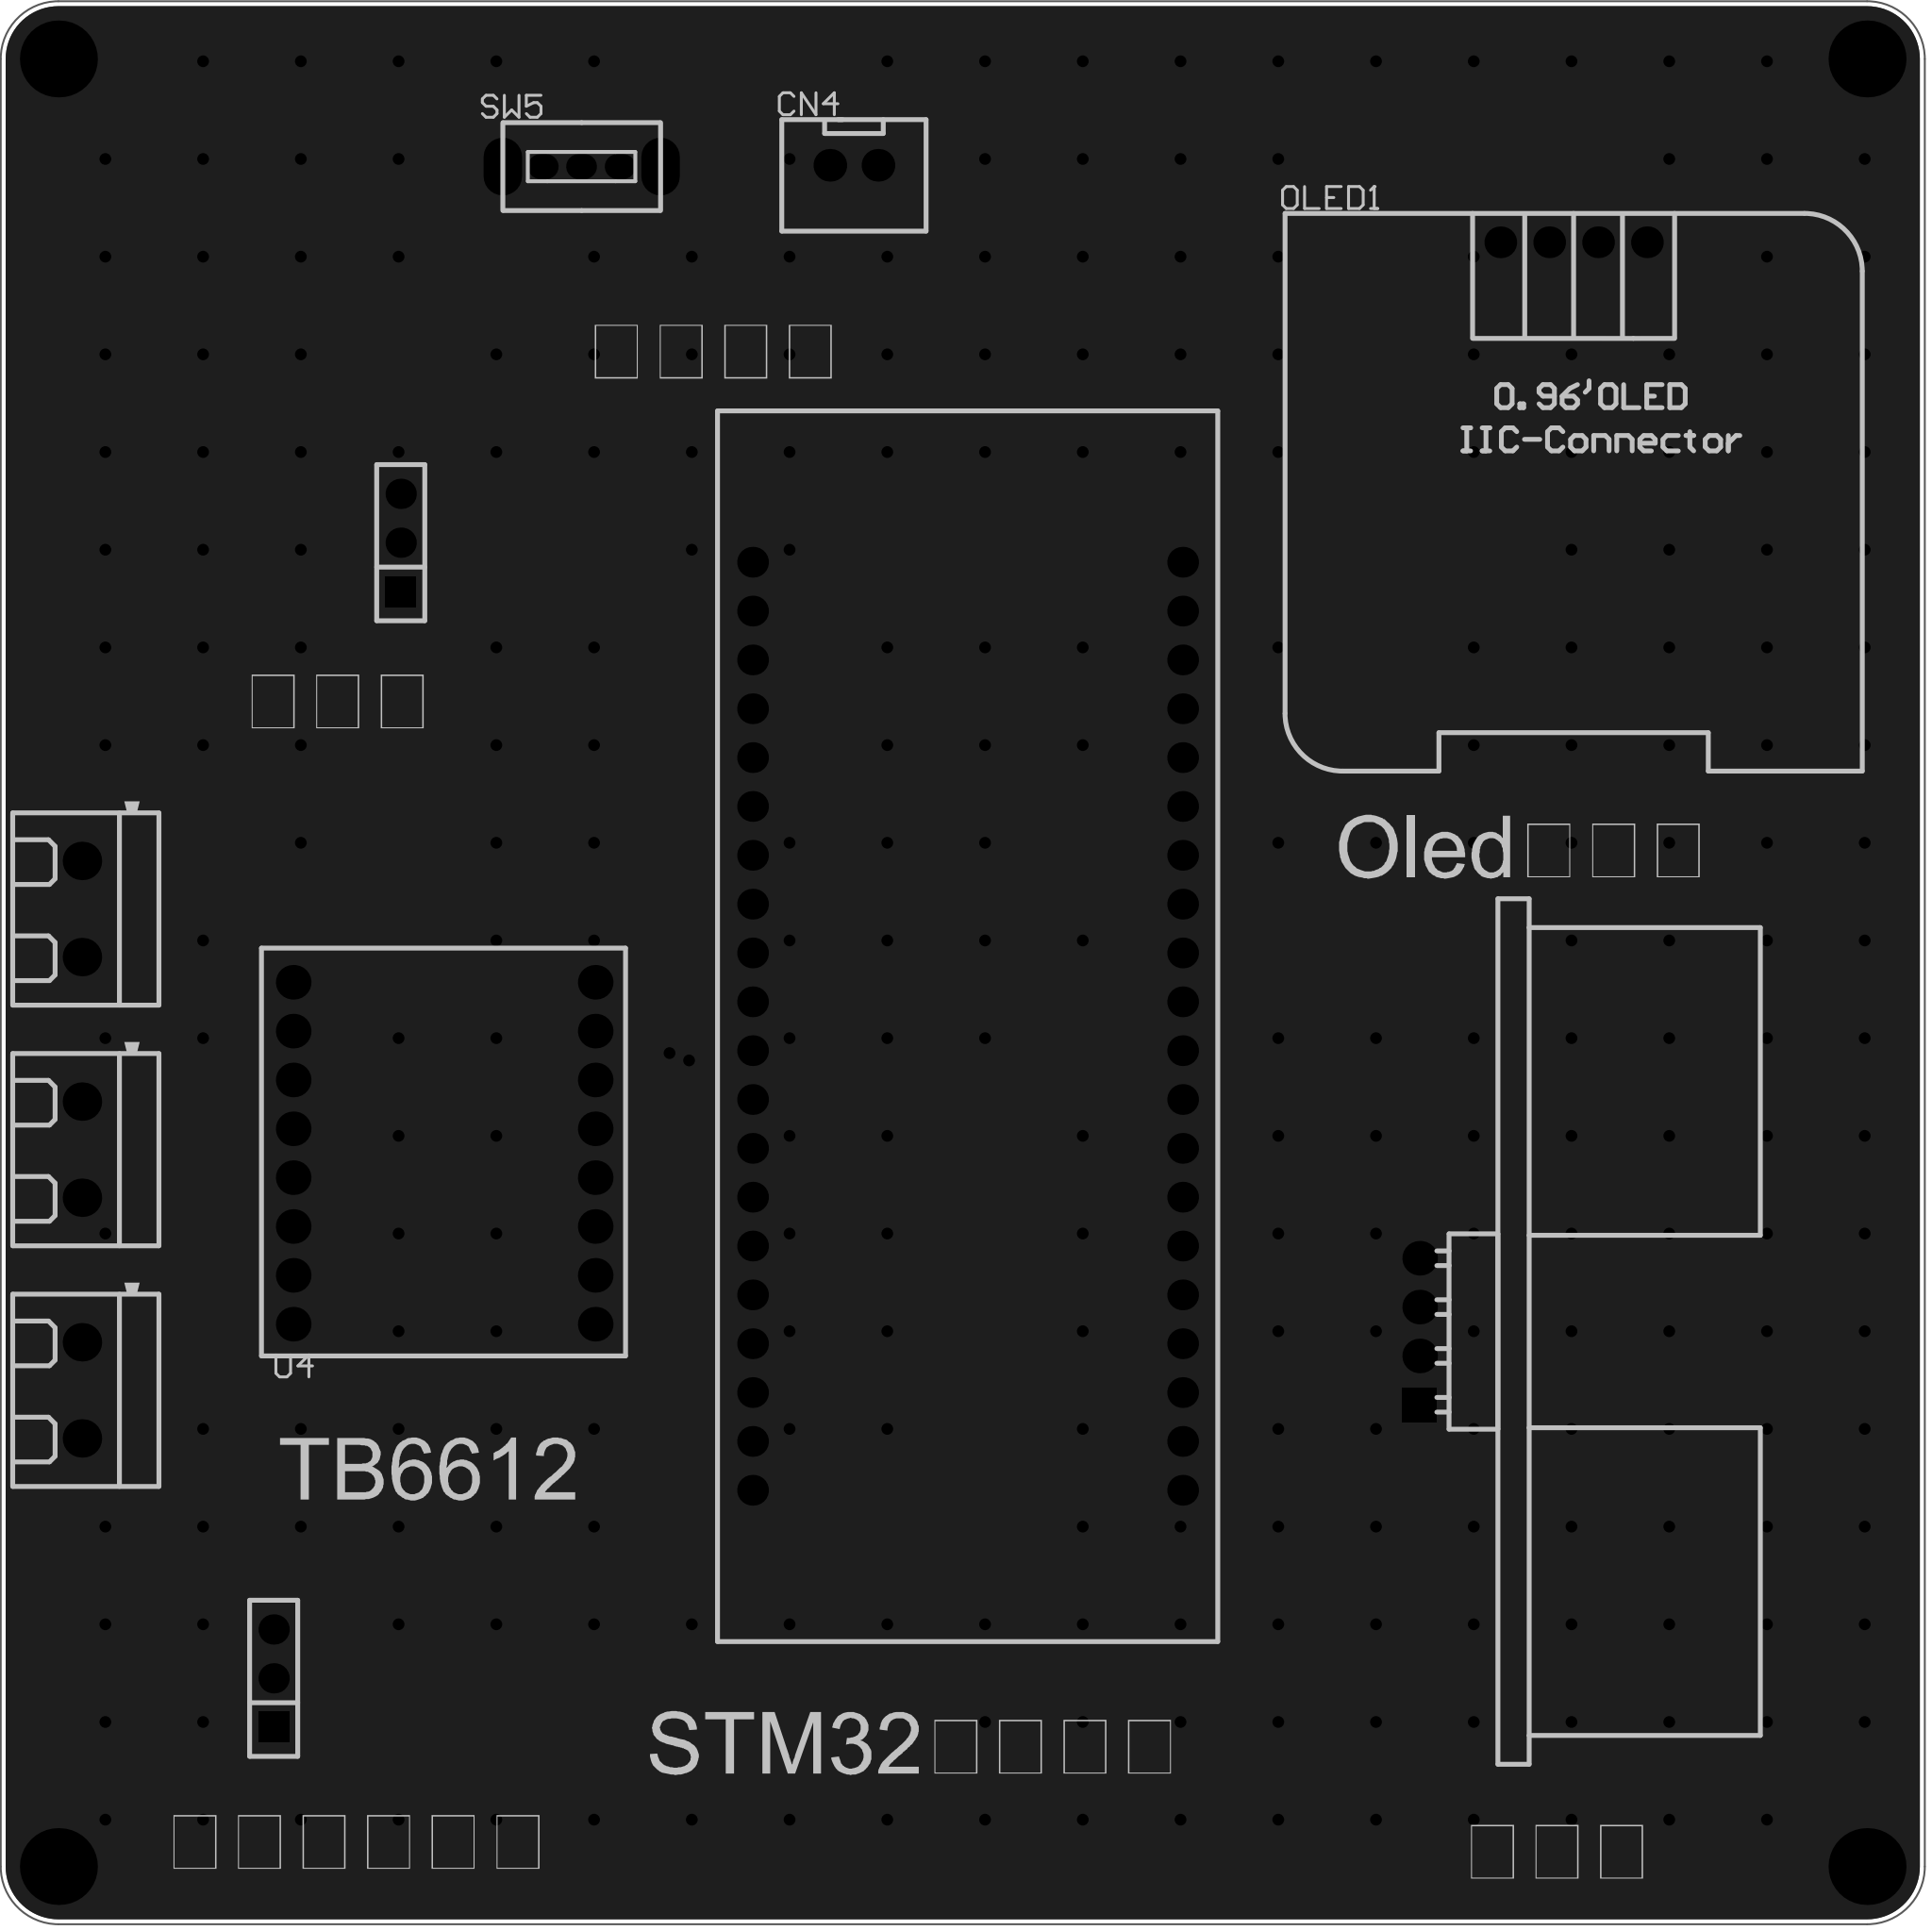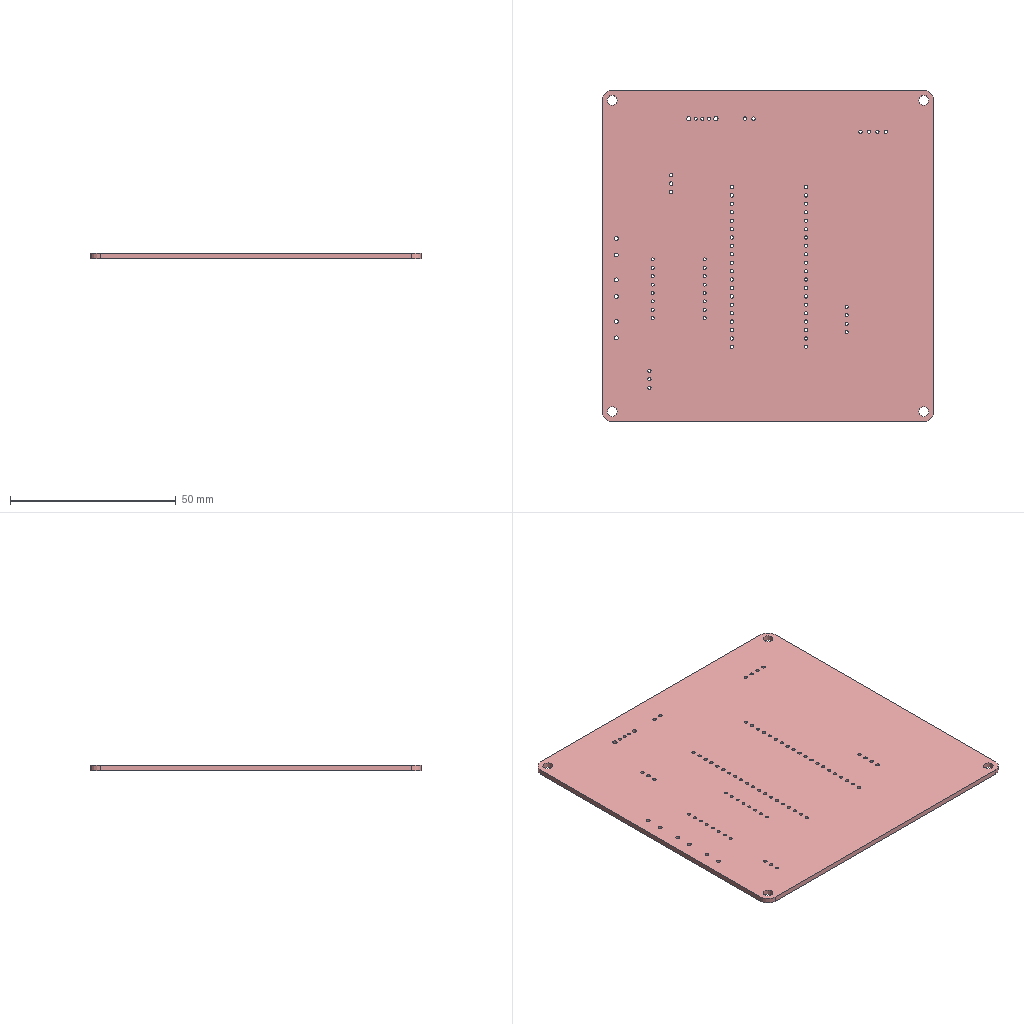Circuit board layout | Altium Designer | box 100 x 100 x 1.6 mm
Layer stack:
# Altium Designer layer stack of  (unit mm; dielectric type: 0 none, 1 core, 2 prepreg, 3 surface material)
index,name,kind,layer,copper_thickness_mm,dielectric_type,dielectric_thickness_mm,dielectric_material,dielectric_constant
0,Top Paste Mask Layer,other,,,,,,
1,Top Silkscreen Layer,other,,,,,,
2,Top Solder Mask Layer,dielectric,,,3,0.01,,3.3
3,Top Layer,copper,Top Layer,0.035,,,,
4,Dielectric1,dielectric,,,3,1.51,FR4,4.5
5,Bottom Layer,copper,Bottom Layer,0.035,,,,
6,Bottom Solder Mask Layer,dielectric,,,3,0.01,,3.3
7,Bottom Silkscreen Layer,other,,,,,,
8,Bottom Paste Mask Layer,other,,,,,,
# drill layer pairs: low layer,high layer
drill_pair,Top Layer,Bottom Layer
Part placement:
Designator,Comment,Layer,Footprint,Center-X(mm),Center-Y(mm),Rotation
U1,STM32F103C8T6-Card,TopLayer,CONN-TH_L53.3-W22.9_STM32F103C8T6-CARD,141.605,127.635,90
H1,,TopLayer,HDR-TH_3P-P2.54-V-F,112.141,152.781,90
H3,,TopLayer,HDR-TH_3P-P2.54-V-F,105.537,93.726,90
OLED1,,TopLayer,0.96OLED_4P,173.101,168.402,0
P1,KF301-2P接线端子,TopLayer,CONN-TH_XY301V-A-5.0-2P,95.574,108.701,90
P2,KF301-2P接线端子,TopLayer,CONN-TH_XY301V-A-5.0-2P,95.574,121.216,90
P3,KF301-2P接线端子,TopLayer,CONN-TH_XY301V-A-5.0-2P,95.574,133.731,90
U2,HC-SR04,TopLayer,TH_HC-SR04V,165.1,111.76,90
U4,,TopLayer,tb6612,114.402,121.031,0
CN4,XH2.54*2P_直插,TopLayer,CONN-TH_2P-P2.50-XH2.54-2P,135.695,172.407,0
SW5,,TopLayer,拨动开关,121.547,172.339,0
Pad and via stacks:
# Altium Designer via and pad stacks of  (unit mm). Each distinct definition once, with the count of objects using it.
# via: kind,start_layer,end_layer,hole_mm,diameter_mm,mode(0 simple;1 top-mid-bottom;2 full stack),diameter_per_layer,count,example_net
# pad: kind,layer,hole_mm,hole_type(0 round;1 square;2 slot),plating,top_size,top_shape(1 round;2 rect;3 octagon;9 rounded rect),mid_size,bottom_size,mode,footprint,size_per_layer,count,example
pad,Multi-Layer,3,0,plated,4x4,1,4x4,4x4,0,,,4,1
pad,Multi-Layer,1,0,plated,1.6x1.6,1,1.6x1.6,1.6x1.6,0,CONN-TH_L53.3-W22.9_STM32F103C8T6-CARD,,40,U1.1
pad,Multi-Layer,1.02,0,plated,1.575x1.575,1,1.575x1.575,1.575x1.575,0,HDR-TH_3P-P2.54-V-F,,4,H1.3
pad,Multi-Layer,1.02,0,plated,1.575x1.575,2,1.575x1.575,1.575x1.575,0,HDR-TH_3P-P2.54-V-F,,2,H1.1
pad,Multi-Layer,1,0,plated,1.65x1.65,1,1.65x1.65,1.65x1.65,0,0.96OLED_4P,,4,OLED1.4
pad,Multi-Layer,1.2,0,plated,2x2,1,2x2,2x2,0,CONN-TH_XY301V-A-5.0-2P,,6,P1.1
pad,Multi-Layer,1.001,0,plated,1.8x1.8,1,1.8x1.8,1.8x1.8,0,TH_HC-SR04V,,3,U2.4
pad,Multi-Layer,1.001,0,plated,1.8x1.8,2,1.8x1.8,1.8x1.8,0,TH_HC-SR04V,,1,U2.1
pad,Multi-Layer,0.9,0,plated,1.8x1.8,1,1.8x1.8,1.8x1.8,0,tb6612,,16,U4.1
pad,Multi-Layer,1.05,0,plated,1.7x1.7,1,1.7x1.7,1.7x1.7,0,CONN-TH_2P-P2.50-XH2.54-2P,,2,CN4.2
pad,Multi-Layer,0.8992,0,plated,1.6x1.3,1,1.6x1.3,1.6x1.3,0,\u00B2\u00A6\u00B6\u00AF\u00BF\u00AA\u00B9\u00D8,,3,SW5.1
pad,Multi-Layer,1.3,0,plated,3x1.999,1,3x1.999,3x1.999,0,\u00B2\u00A6\u00B6\u00AF\u00BF\u00AA\u00B9\u00D8,,2,SW5.4
via,Top Layer,Bottom Layer,0.3048,0.61,0,,268,PB0
Copper pours:
name,layer,net,type(0 solid;1 hatched;2 none)
Bottom Layer-GND,Bottom Layer,GND,0
Top Layer-GND,Top Layer,GND,0
Design rules, without the lines most boards share:
# Altium Designer design rules of  (exported by Altium Designer, unit mm)
# columns: name | kind | enabled | priority | scope1 | scope2 | descriptor | typed fields (field=value)
Copper_copperRegion_copperThickness1oz | 0 | disabled | 4 | All | All | Clearance Constraint (Gap=5.984mil) (Disabled)(All),(All) | gap=0.152
Copper_copperRegion_copperThickness1oz_1 | 63 | disabled | 4 | All | All | Board Clearance Constraint (Gap=0mil) (Disabled)(All) |
Copper_copperRegion_Copper_copperRegion | 0 | disabled | 5 | All | All | Clearance Constraint (Gap=5.984mil) (Disabled)(All),(All) | gap=0.152
Copper_copperRegion_Copper_copperRegion_1 | 63 | disabled | 5 | All | All | Board Clearance Constraint (Gap=0mil) (Disabled)(All) |
copperThickness1oz | 0 | enabled | 6 | All | All | Clearance Constraint (Gap=5.984mil) (All),(All) | gap=0.152
copperThickness1oz_1 | 63 | enabled | 6 | All | All | Board Clearance Constraint (Gap=0mil) (All) |
copperRegion_copperThickness1oz | 20 | disabled | 1 | All | All | Polygon Connect Rule(Relief Connect )(Conductor Width=10mil) (Relief Angle=90 Angle) (Entries=4) (Air Gap Width=10mil) (Disabled)(All),(All) | connect_style(0=relief,1=direct,2=none)=0 relief_conductor_width=0.254 relief_entries=4
copperRegion_Copper_copperRegion | 20 | disabled | 2 | All | All | Polygon Connect Rule(Relief Connect )(Conductor Width=10mil) (Relief Angle=90 Angle) (Entries=4) (Air Gap Width=10mil) (Disabled)(All),(All) | connect_style(0=relief,1=direct,2=none)=0 relief_conductor_width=0.254 relief_entries=4
copperRegion | 20 | enabled | 3 | All | All | Polygon Connect Rule(Relief Connect )(Conductor Width=10mil) (Relief Angle=90 Angle) (Entries=4) (Air Gap Width=10mil) (All),(All) | connect_style(0=relief,1=direct,2=none)=0 relief_conductor_width=0.254 relief_entries=4